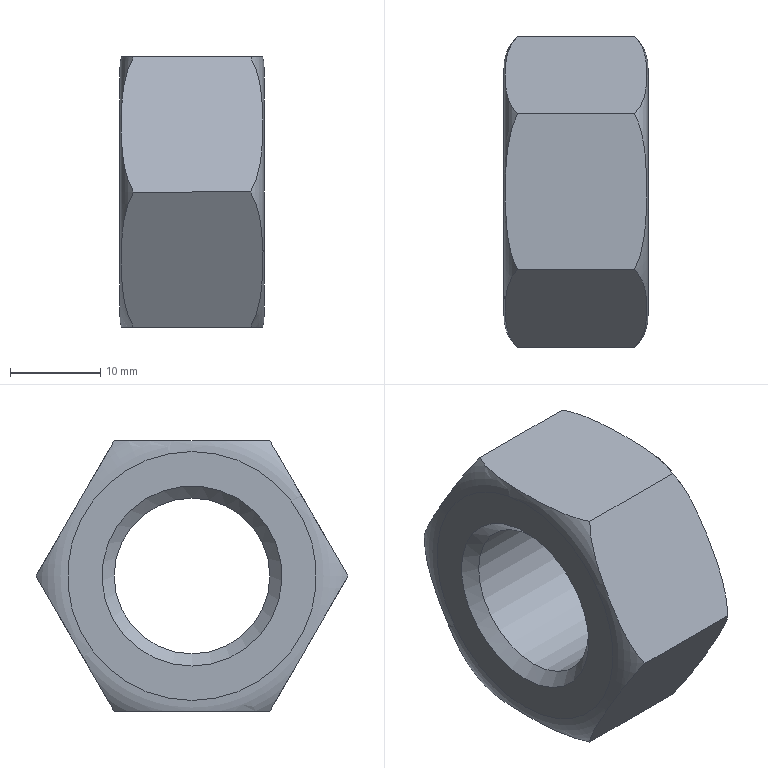Part | STEP file | C-CFJFNV60-20-150_n | 1 solid | 13 faces | box 16 x 34.641 x 30 mm | volume 8537 mm3 | plane 8 | torus 2 | cone 2 | cylinder 1 | commonest cylinder face diameters 17.294 x1
STEP:
#1=CARTESIAN_POINT('',(-6.5,8.66,15.));
#2=VERTEX_POINT('',#1);
#3=CARTESIAN_POINT('',(-7.854,0.,15.));
#4=VERTEX_POINT('',#3);
#5=CARTESIAN_POINT('',(-6.5,8.66,15.));
#6=CARTESIAN_POINT('',(-6.609,8.453,15.));
#7=CARTESIAN_POINT('',(-6.705,8.244,15.));
#8=CARTESIAN_POINT('',(-7.285,6.855,15.));
#9=CARTESIAN_POINT('',(-7.54,5.487,15.));
#10=CARTESIAN_POINT('',(-7.821,2.703,15.));
#11=CARTESIAN_POINT('',(-7.854,1.288,15.));
#12=CARTESIAN_POINT('',(-7.854,0.,15.));
#13=B_SPLINE_CURVE_WITH_KNOTS('',3,(#5,#6,#7,#8,#9,#10,#11,#12),.UNSPECIFIED.,.F.,.F.,(4,2,2,4),(4.146,4.211,4.598,4.984),.UNSPECIFIED.);
#14=EDGE_CURVE('',#2,#4,#13,.T.);
#15=ORIENTED_EDGE('',*,*,#14,.F.);
#16=CARTESIAN_POINT('',(-6.5,17.321,0.));
#17=VERTEX_POINT('',#16);
#18=CARTESIAN_POINT('',(-6.5,17.321,0.));
#19=CARTESIAN_POINT('',(-6.609,17.217,0.1798));
#20=CARTESIAN_POINT('',(-6.705,17.112,0.3609));
#21=CARTESIAN_POINT('',(-7.285,16.418,1.564));
#22=CARTESIAN_POINT('',(-7.54,15.734,2.748));
#23=CARTESIAN_POINT('',(-7.821,14.342,5.159));
#24=CARTESIAN_POINT('',(-7.854,13.634,6.385));
#25=CARTESIAN_POINT('',(-7.854,12.99,7.5));
#26=CARTESIAN_POINT('',(-7.854,12.346,8.615));
#27=CARTESIAN_POINT('',(-7.821,11.639,9.841));
#28=CARTESIAN_POINT('',(-7.54,10.247,12.252));
#29=CARTESIAN_POINT('',(-7.285,9.563,13.436));
#30=CARTESIAN_POINT('',(-6.705,8.869,14.639));
#31=CARTESIAN_POINT('',(-6.609,8.764,14.82));
#32=CARTESIAN_POINT('',(-6.5,8.66,15.));
#33=B_SPLINE_CURVE_WITH_KNOTS('',3,(#18,#19,#20,#21,#22,#23,#24,#25,#26,#27,#28,#29,#30,#31,#32),.UNSPECIFIED.,.F.,.F.,(4,2,2,3,2,2,4),(4.146,4.211,4.598,4.984,5.37,5.757,5.822),.UNSPECIFIED.);
#34=EDGE_CURVE('',#17,#2,#33,.T.);
#35=ORIENTED_EDGE('',*,*,#34,.F.);
#36=CARTESIAN_POINT('',(-6.5,8.66,-15.));
#37=VERTEX_POINT('',#36);
#38=CARTESIAN_POINT('',(-6.5,8.66,-15.));
#39=CARTESIAN_POINT('',(-6.609,8.764,-14.82));
#40=CARTESIAN_POINT('',(-6.705,8.869,-14.639));
#41=CARTESIAN_POINT('',(-7.285,9.563,-13.436));
#42=CARTESIAN_POINT('',(-7.54,10.247,-12.252));
#43=CARTESIAN_POINT('',(-7.821,11.639,-9.841));
#44=CARTESIAN_POINT('',(-7.854,12.346,-8.615));
#45=CARTESIAN_POINT('',(-7.854,12.99,-7.5));
#46=CARTESIAN_POINT('',(-7.854,13.634,-6.385));
#47=CARTESIAN_POINT('',(-7.821,14.342,-5.159));
#48=CARTESIAN_POINT('',(-7.54,15.734,-2.748));
#49=CARTESIAN_POINT('',(-7.285,16.418,-1.564));
#50=CARTESIAN_POINT('',(-6.705,17.112,-0.3609));
#51=CARTESIAN_POINT('',(-6.609,17.217,-0.1798));
#52=CARTESIAN_POINT('',(-6.5,17.321,0.));
#53=B_SPLINE_CURVE_WITH_KNOTS('',3,(#38,#39,#40,#41,#42,#43,#44,#45,#46,#47,#48,#49,#50,#51,#52),.UNSPECIFIED.,.F.,.F.,(4,2,2,3,2,2,4),(4.146,4.211,4.598,4.984,5.37,5.757,5.822),.UNSPECIFIED.);
#54=EDGE_CURVE('',#37,#17,#53,.T.);
#55=ORIENTED_EDGE('',*,*,#54,.F.);
#56=CARTESIAN_POINT('',(-6.5,-8.66,-15.));
#57=VERTEX_POINT('',#56);
#58=CARTESIAN_POINT('',(-6.5,-8.66,-15.));
#59=CARTESIAN_POINT('',(-6.609,-8.453,-15.));
#60=CARTESIAN_POINT('',(-6.705,-8.244,-15.));
#61=CARTESIAN_POINT('',(-7.285,-6.855,-15.));
#62=CARTESIAN_POINT('',(-7.54,-5.487,-15.));
#63=CARTESIAN_POINT('',(-7.821,-2.703,-15.));
#64=CARTESIAN_POINT('',(-7.854,-1.288,-15.));
#65=CARTESIAN_POINT('',(-7.854,0.,-15.));
#66=CARTESIAN_POINT('',(-7.854,1.288,-15.));
#67=CARTESIAN_POINT('',(-7.821,2.703,-15.));
#68=CARTESIAN_POINT('',(-7.54,5.487,-15.));
#69=CARTESIAN_POINT('',(-7.285,6.855,-15.));
#70=CARTESIAN_POINT('',(-6.705,8.244,-15.));
#71=CARTESIAN_POINT('',(-6.609,8.453,-15.));
#72=CARTESIAN_POINT('',(-6.5,8.66,-15.));
#73=B_SPLINE_CURVE_WITH_KNOTS('',3,(#58,#59,#60,#61,#62,#63,#64,#65,#66,#67,#68,#69,#70,#71,#72),.UNSPECIFIED.,.F.,.F.,(4,2,2,3,2,2,4),(4.146,4.211,4.598,4.984,5.37,5.757,5.822),.UNSPECIFIED.);
#74=EDGE_CURVE('',#57,#37,#73,.T.);
#75=ORIENTED_EDGE('',*,*,#74,.F.);
#76=CARTESIAN_POINT('',(-6.5,-17.321,0.));
#77=VERTEX_POINT('',#76);
#78=CARTESIAN_POINT('',(-6.5,-17.321,0.));
#79=CARTESIAN_POINT('',(-6.609,-17.217,-0.1798));
#80=CARTESIAN_POINT('',(-6.705,-17.112,-0.3609));
#81=CARTESIAN_POINT('',(-7.285,-16.418,-1.564));
#82=CARTESIAN_POINT('',(-7.54,-15.734,-2.748));
#83=CARTESIAN_POINT('',(-7.821,-14.342,-5.159));
#84=CARTESIAN_POINT('',(-7.854,-13.634,-6.385));
#85=CARTESIAN_POINT('',(-7.854,-12.99,-7.5));
#86=CARTESIAN_POINT('',(-7.854,-12.346,-8.615));
#87=CARTESIAN_POINT('',(-7.821,-11.639,-9.841));
#88=CARTESIAN_POINT('',(-7.54,-10.247,-12.252));
#89=CARTESIAN_POINT('',(-7.285,-9.563,-13.436));
#90=CARTESIAN_POINT('',(-6.705,-8.869,-14.639));
#91=CARTESIAN_POINT('',(-6.609,-8.764,-14.82));
#92=CARTESIAN_POINT('',(-6.5,-8.66,-15.));
#93=B_SPLINE_CURVE_WITH_KNOTS('',3,(#78,#79,#80,#81,#82,#83,#84,#85,#86,#87,#88,#89,#90,#91,#92),.UNSPECIFIED.,.F.,.F.,(4,2,2,3,2,2,4),(4.146,4.211,4.598,4.984,5.37,5.757,5.822),.UNSPECIFIED.);
#94=EDGE_CURVE('',#77,#57,#93,.T.);
#95=ORIENTED_EDGE('',*,*,#94,.F.);
#96=CARTESIAN_POINT('',(-6.5,-8.66,15.));
#97=VERTEX_POINT('',#96);
#98=CARTESIAN_POINT('',(-6.5,-8.66,15.));
#99=CARTESIAN_POINT('',(-6.609,-8.764,14.82));
#100=CARTESIAN_POINT('',(-6.705,-8.869,14.639));
#101=CARTESIAN_POINT('',(-7.285,-9.563,13.436));
#102=CARTESIAN_POINT('',(-7.54,-10.247,12.252));
#103=CARTESIAN_POINT('',(-7.821,-11.639,9.841));
#104=CARTESIAN_POINT('',(-7.854,-12.346,8.615));
#105=CARTESIAN_POINT('',(-7.854,-12.99,7.5));
#106=CARTESIAN_POINT('',(-7.854,-13.634,6.385));
#107=CARTESIAN_POINT('',(-7.821,-14.342,5.159));
#108=CARTESIAN_POINT('',(-7.54,-15.734,2.748));
#109=CARTESIAN_POINT('',(-7.285,-16.418,1.564));
#110=CARTESIAN_POINT('',(-6.705,-17.112,0.3609));
#111=CARTESIAN_POINT('',(-6.609,-17.217,0.1798));
#112=CARTESIAN_POINT('',(-6.5,-17.321,0.));
#113=B_SPLINE_CURVE_WITH_KNOTS('',3,(#98,#99,#100,#101,#102,#103,#104,#105,#106,#107,#108,#109,#110,#111,#112),.UNSPECIFIED.,.F.,.F.,(4,2,2,3,2,2,4),(4.146,4.211,4.598,4.984,5.37,5.757,5.822),.UNSPECIFIED.);
#114=EDGE_CURVE('',#97,#77,#113,.T.);
#115=ORIENTED_EDGE('',*,*,#114,.F.);
#116=CARTESIAN_POINT('',(-7.854,0.,15.));
#117=CARTESIAN_POINT('',(-7.854,-1.288,15.));
#118=CARTESIAN_POINT('',(-7.821,-2.703,15.));
#119=CARTESIAN_POINT('',(-7.54,-5.487,15.));
#120=CARTESIAN_POINT('',(-7.285,-6.855,15.));
#121=CARTESIAN_POINT('',(-6.705,-8.244,15.));
#122=CARTESIAN_POINT('',(-6.609,-8.453,15.));
#123=CARTESIAN_POINT('',(-6.5,-8.66,15.));
#124=B_SPLINE_CURVE_WITH_KNOTS('',3,(#116,#117,#118,#119,#120,#121,#122,#123),.UNSPECIFIED.,.F.,.F.,(4,2,2,4),(4.984,5.37,5.757,5.822),.UNSPECIFIED.);
#125=EDGE_CURVE('',#4,#97,#124,.T.);
#126=ORIENTED_EDGE('',*,*,#125,.F.);
#127=CARTESIAN_POINT('',(-8.,0.,13.821));
#128=VERTEX_POINT('',#127);
#129=CARTESIAN_POINT('',(-3.167,0.,13.821));
#130=DIRECTION('',(0.,-1.,0.));
#131=DIRECTION('',(0.,0.,1.));
#132=AXIS2_PLACEMENT_3D('',#129,#130,#131);
#133=CIRCLE('',#132,4.833);
#134=EDGE_CURVE('',#4,#128,#133,.T.);
#135=ORIENTED_EDGE('',*,*,#134,.T.);
#136=CARTESIAN_POINT('',(-8.,0.,-13.821));
#137=VERTEX_POINT('',#136);
#138=CARTESIAN_POINT('',(-8.,0.,0.));
#139=DIRECTION('',(1.,0.,0.));
#140=DIRECTION('',(0.,0.,-1.));
#141=AXIS2_PLACEMENT_3D('',#138,#139,#140);
#142=CIRCLE('',#141,13.821);
#143=EDGE_CURVE('',#128,#137,#142,.T.);
#144=ORIENTED_EDGE('',*,*,#143,.T.);
#145=CARTESIAN_POINT('',(-8.,0.,0.));
#146=DIRECTION('',(1.,0.,0.));
#147=DIRECTION('',(0.,0.,-1.));
#148=AXIS2_PLACEMENT_3D('',#145,#146,#147);
#149=CIRCLE('',#148,13.821);
#150=EDGE_CURVE('',#137,#128,#149,.T.);
#151=ORIENTED_EDGE('',*,*,#150,.T.);
#152=ORIENTED_EDGE('',*,*,#134,.F.);
#153=EDGE_LOOP('',(#15,#35,#55,#75,#95,#115,#126,#135,#144,#151,#152));
#154=FACE_OUTER_BOUND('',#153,.T.);
#155=CARTESIAN_POINT('',(-3.167,0.,0.));
#156=DIRECTION('',(1.,0.,0.));
#157=DIRECTION('',(0.,0.,-1.));
#158=AXIS2_PLACEMENT_3D('',#155,#156,#157);
#159=TOROIDAL_SURFACE('',#158,13.821,4.833);
#160=ADVANCED_FACE('',(#154),#159,.T.);
#161=ORIENTED_EDGE('',*,*,#150,.F.);
#162=ORIENTED_EDGE('',*,*,#143,.F.);
#163=EDGE_LOOP('',(#161,#162));
#164=FACE_OUTER_BOUND('',#163,.T.);
#165=CARTESIAN_POINT('',(-8.,0.,-10.));
#166=VERTEX_POINT('',#165);
#167=CARTESIAN_POINT('',(-8.,0.,0.));
#168=DIRECTION('',(1.,0.,0.));
#169=DIRECTION('',(0.,0.,-1.));
#170=AXIS2_PLACEMENT_3D('',#167,#168,#169);
#171=CIRCLE('',#170,10.);
#172=EDGE_CURVE('',#166,#166,#171,.T.);
#173=ORIENTED_EDGE('',*,*,#172,.T.);
#174=EDGE_LOOP('',(#173));
#175=FACE_BOUND('',#174,.T.);
#176=CARTESIAN_POINT('',(-8.,13.821,0.));
#177=DIRECTION('',(-1.,0.,0.));
#178=DIRECTION('',(0.,0.,1.));
#179=AXIS2_PLACEMENT_3D('',#176,#177,#178);
#180=PLANE('',#179);
#181=ADVANCED_FACE('',(#164,#175),#180,.T.);
#182=CARTESIAN_POINT('',(-6.647,0.,-8.647));
#183=VERTEX_POINT('',#182);
#184=CARTESIAN_POINT('',(-6.647,0.,8.647));
#185=VERTEX_POINT('',#184);
#186=CARTESIAN_POINT('',(-6.647,0.,0.));
#187=DIRECTION('',(1.,0.,0.));
#188=DIRECTION('',(0.,0.,-1.));
#189=AXIS2_PLACEMENT_3D('',#186,#187,#188);
#190=CIRCLE('',#189,8.647);
#191=EDGE_CURVE('',#183,#185,#190,.T.);
#192=ORIENTED_EDGE('',*,*,#191,.T.);
#193=CARTESIAN_POINT('',(-6.647,0.,0.));
#194=DIRECTION('',(1.,0.,0.));
#195=DIRECTION('',(0.,0.,-1.));
#196=AXIS2_PLACEMENT_3D('',#193,#194,#195);
#197=CIRCLE('',#196,8.647);
#198=EDGE_CURVE('',#185,#183,#197,.T.);
#199=ORIENTED_EDGE('',*,*,#198,.T.);
#200=CARTESIAN_POINT('',(-8.,0.,-10.));
#201=DIRECTION('',(-0.7071,0.,-0.7071));
#202=VECTOR('',#201,10.);
#203=LINE('',#200,#202);
#204=EDGE_CURVE('',#183,#166,#203,.T.);
#205=ORIENTED_EDGE('',*,*,#204,.T.);
#206=ORIENTED_EDGE('',*,*,#172,.F.);
#207=ORIENTED_EDGE('',*,*,#204,.F.);
#208=EDGE_LOOP('',(#192,#199,#205,#206,#207));
#209=FACE_OUTER_BOUND('',#208,.T.);
#210=CARTESIAN_POINT('',(-8.,0.,0.));
#211=DIRECTION('',(-1.,0.,0.));
#212=DIRECTION('',(0.,0.,1.));
#213=AXIS2_PLACEMENT_3D('',#210,#211,#212);
#214=CONICAL_SURFACE('',#213,10.,0.7854);
#215=ADVANCED_FACE('',(#209),#214,.F.);
#216=ORIENTED_EDGE('',*,*,#191,.F.);
#217=ORIENTED_EDGE('',*,*,#198,.F.);
#218=CARTESIAN_POINT('',(6.647,0.,8.647));
#219=VERTEX_POINT('',#218);
#220=CARTESIAN_POINT('',(8.,0.,8.647));
#221=DIRECTION('',(1.,0.,0.));
#222=VECTOR('',#221,8.647);
#223=LINE('',#220,#222);
#224=EDGE_CURVE('',#185,#219,#223,.T.);
#225=ORIENTED_EDGE('',*,*,#224,.T.);
#226=CARTESIAN_POINT('',(6.647,0.,-8.647));
#227=VERTEX_POINT('',#226);
#228=CARTESIAN_POINT('',(6.647,0.,0.));
#229=DIRECTION('',(1.,0.,0.));
#230=DIRECTION('',(0.,0.,-1.));
#231=AXIS2_PLACEMENT_3D('',#228,#229,#230);
#232=CIRCLE('',#231,8.647);
#233=EDGE_CURVE('',#219,#227,#232,.T.);
#234=ORIENTED_EDGE('',*,*,#233,.T.);
#235=CARTESIAN_POINT('',(6.647,0.,0.));
#236=DIRECTION('',(1.,0.,0.));
#237=DIRECTION('',(0.,0.,-1.));
#238=AXIS2_PLACEMENT_3D('',#235,#236,#237);
#239=CIRCLE('',#238,8.647);
#240=EDGE_CURVE('',#227,#219,#239,.T.);
#241=ORIENTED_EDGE('',*,*,#240,.T.);
#242=ORIENTED_EDGE('',*,*,#224,.F.);
#243=EDGE_LOOP('',(#216,#217,#225,#234,#241,#242));
#244=FACE_OUTER_BOUND('',#243,.T.);
#245=CARTESIAN_POINT('',(8.,0.,0.));
#246=DIRECTION('',(1.,0.,0.));
#247=DIRECTION('',(0.,0.,-1.));
#248=AXIS2_PLACEMENT_3D('',#245,#246,#247);
#249=CYLINDRICAL_SURFACE('',#248,8.647);
#250=ADVANCED_FACE('',(#244),#249,.F.);
#251=ORIENTED_EDGE('',*,*,#240,.F.);
#252=ORIENTED_EDGE('',*,*,#233,.F.);
#253=CARTESIAN_POINT('',(8.,0.,10.));
#254=VERTEX_POINT('',#253);
#255=CARTESIAN_POINT('',(6.647,0.,8.647));
#256=DIRECTION('',(0.7071,0.,0.7071));
#257=VECTOR('',#256,8.647);
#258=LINE('',#255,#257);
#259=EDGE_CURVE('',#219,#254,#258,.T.);
#260=ORIENTED_EDGE('',*,*,#259,.T.);
#261=CARTESIAN_POINT('',(8.,0.,-10.));
#262=VERTEX_POINT('',#261);
#263=CARTESIAN_POINT('',(8.,0.,0.));
#264=DIRECTION('',(1.,0.,0.));
#265=DIRECTION('',(0.,0.,-1.));
#266=AXIS2_PLACEMENT_3D('',#263,#264,#265);
#267=CIRCLE('',#266,10.);
#268=EDGE_CURVE('',#254,#262,#267,.T.);
#269=ORIENTED_EDGE('',*,*,#268,.T.);
#270=CARTESIAN_POINT('',(8.,0.,0.));
#271=DIRECTION('',(1.,0.,0.));
#272=DIRECTION('',(0.,0.,-1.));
#273=AXIS2_PLACEMENT_3D('',#270,#271,#272);
#274=CIRCLE('',#273,10.);
#275=EDGE_CURVE('',#262,#254,#274,.T.);
#276=ORIENTED_EDGE('',*,*,#275,.T.);
#277=ORIENTED_EDGE('',*,*,#259,.F.);
#278=EDGE_LOOP('',(#251,#252,#260,#269,#276,#277));
#279=FACE_OUTER_BOUND('',#278,.T.);
#280=CARTESIAN_POINT('',(6.647,0.,0.));
#281=DIRECTION('',(1.,0.,0.));
#282=DIRECTION('',(0.,0.,-1.));
#283=AXIS2_PLACEMENT_3D('',#280,#281,#282);
#284=CONICAL_SURFACE('',#283,8.647,0.7854);
#285=ADVANCED_FACE('',(#279),#284,.F.);
#286=CARTESIAN_POINT('',(8.,0.,-13.821));
#287=VERTEX_POINT('',#286);
#288=CARTESIAN_POINT('',(8.,0.,13.821));
#289=VERTEX_POINT('',#288);
#290=CARTESIAN_POINT('',(8.,0.,0.));
#291=DIRECTION('',(1.,0.,0.));
#292=DIRECTION('',(0.,0.,-1.));
#293=AXIS2_PLACEMENT_3D('',#290,#291,#292);
#294=CIRCLE('',#293,13.821);
#295=EDGE_CURVE('',#287,#289,#294,.T.);
#296=ORIENTED_EDGE('',*,*,#295,.T.);
#297=CARTESIAN_POINT('',(8.,0.,0.));
#298=DIRECTION('',(1.,0.,0.));
#299=DIRECTION('',(0.,0.,-1.));
#300=AXIS2_PLACEMENT_3D('',#297,#298,#299);
#301=CIRCLE('',#300,13.821);
#302=EDGE_CURVE('',#289,#287,#301,.T.);
#303=ORIENTED_EDGE('',*,*,#302,.T.);
#304=EDGE_LOOP('',(#296,#303));
#305=FACE_OUTER_BOUND('',#304,.T.);
#306=ORIENTED_EDGE('',*,*,#275,.F.);
#307=ORIENTED_EDGE('',*,*,#268,.F.);
#308=EDGE_LOOP('',(#306,#307));
#309=FACE_BOUND('',#308,.T.);
#310=CARTESIAN_POINT('',(8.,10.,0.));
#311=DIRECTION('',(1.,0.,0.));
#312=DIRECTION('',(0.,0.,-1.));
#313=AXIS2_PLACEMENT_3D('',#310,#311,#312);
#314=PLANE('',#313);
#315=ADVANCED_FACE('',(#305,#309),#314,.T.);
#316=ORIENTED_EDGE('',*,*,#295,.F.);
#317=ORIENTED_EDGE('',*,*,#302,.F.);
#318=CARTESIAN_POINT('',(7.854,0.,15.));
#319=VERTEX_POINT('',#318);
#320=CARTESIAN_POINT('',(3.167,0.,13.821));
#321=DIRECTION('',(0.,-1.,0.));
#322=DIRECTION('',(0.,0.,1.));
#323=AXIS2_PLACEMENT_3D('',#320,#321,#322);
#324=CIRCLE('',#323,4.833);
#325=EDGE_CURVE('',#289,#319,#324,.T.);
#326=ORIENTED_EDGE('',*,*,#325,.T.);
#327=CARTESIAN_POINT('',(6.5,-8.66,15.));
#328=VERTEX_POINT('',#327);
#329=CARTESIAN_POINT('',(6.5,-8.66,15.));
#330=CARTESIAN_POINT('',(6.609,-8.453,15.));
#331=CARTESIAN_POINT('',(6.705,-8.244,15.));
#332=CARTESIAN_POINT('',(7.285,-6.855,15.));
#333=CARTESIAN_POINT('',(7.54,-5.487,15.));
#334=CARTESIAN_POINT('',(7.821,-2.703,15.));
#335=CARTESIAN_POINT('',(7.854,-1.288,15.));
#336=CARTESIAN_POINT('',(7.854,0.,15.));
#337=B_SPLINE_CURVE_WITH_KNOTS('',3,(#329,#330,#331,#332,#333,#334,#335,#336),.UNSPECIFIED.,.F.,.F.,(4,2,2,4),(1.654,1.719,2.106,2.492),.UNSPECIFIED.);
#338=EDGE_CURVE('',#328,#319,#337,.T.);
#339=ORIENTED_EDGE('',*,*,#338,.F.);
#340=CARTESIAN_POINT('',(6.5,-17.321,0.));
#341=VERTEX_POINT('',#340);
#342=CARTESIAN_POINT('',(6.5,-17.321,0.));
#343=CARTESIAN_POINT('',(6.609,-17.217,0.1798));
#344=CARTESIAN_POINT('',(6.705,-17.112,0.3609));
#345=CARTESIAN_POINT('',(7.285,-16.418,1.564));
#346=CARTESIAN_POINT('',(7.54,-15.734,2.748));
#347=CARTESIAN_POINT('',(7.821,-14.342,5.159));
#348=CARTESIAN_POINT('',(7.854,-13.634,6.385));
#349=CARTESIAN_POINT('',(7.854,-12.346,8.615));
#350=CARTESIAN_POINT('',(7.821,-11.639,9.841));
#351=CARTESIAN_POINT('',(7.54,-10.247,12.252));
#352=CARTESIAN_POINT('',(7.285,-9.563,13.436));
#353=CARTESIAN_POINT('',(6.705,-8.869,14.639));
#354=CARTESIAN_POINT('',(6.609,-8.764,14.82));
#355=CARTESIAN_POINT('',(6.5,-8.66,15.));
#356=B_SPLINE_CURVE_WITH_KNOTS('',3,(#342,#343,#344,#345,#346,#347,#348,#349,#350,#351,#352,#353,#354,#355),.UNSPECIFIED.,.F.,.F.,(4,2,2,2,2,2,4),(1.654,1.719,2.106,2.492,2.878,3.265,3.33),.UNSPECIFIED.);
#357=EDGE_CURVE('',#341,#328,#356,.T.);
#358=ORIENTED_EDGE('',*,*,#357,.F.);
#359=CARTESIAN_POINT('',(6.5,-8.66,-15.));
#360=VERTEX_POINT('',#359);
#361=CARTESIAN_POINT('',(6.5,-8.66,-15.));
#362=CARTESIAN_POINT('',(6.609,-8.764,-14.82));
#363=CARTESIAN_POINT('',(6.705,-8.869,-14.639));
#364=CARTESIAN_POINT('',(7.285,-9.563,-13.436));
#365=CARTESIAN_POINT('',(7.54,-10.247,-12.252));
#366=CARTESIAN_POINT('',(7.821,-11.639,-9.841));
#367=CARTESIAN_POINT('',(7.854,-12.346,-8.615));
#368=CARTESIAN_POINT('',(7.854,-13.634,-6.385));
#369=CARTESIAN_POINT('',(7.821,-14.342,-5.159));
#370=CARTESIAN_POINT('',(7.54,-15.734,-2.748));
#371=CARTESIAN_POINT('',(7.285,-16.418,-1.564));
#372=CARTESIAN_POINT('',(6.705,-17.112,-0.3609));
#373=CARTESIAN_POINT('',(6.609,-17.217,-0.1798));
#374=CARTESIAN_POINT('',(6.5,-17.321,0.));
#375=B_SPLINE_CURVE_WITH_KNOTS('',3,(#361,#362,#363,#364,#365,#366,#367,#368,#369,#370,#371,#372,#373,#374),.UNSPECIFIED.,.F.,.F.,(4,2,2,2,2,2,4),(1.654,1.719,2.106,2.492,2.878,3.265,3.33),.UNSPECIFIED.);
#376=EDGE_CURVE('',#360,#341,#375,.T.);
#377=ORIENTED_EDGE('',*,*,#376,.F.);
#378=CARTESIAN_POINT('',(6.5,8.66,-15.));
#379=VERTEX_POINT('',#378);
#380=CARTESIAN_POINT('',(6.5,8.66,-15.));
#381=CARTESIAN_POINT('',(6.609,8.453,-15.));
#382=CARTESIAN_POINT('',(6.705,8.244,-15.));
#383=CARTESIAN_POINT('',(7.285,6.855,-15.));
#384=CARTESIAN_POINT('',(7.54,5.487,-15.));
#385=CARTESIAN_POINT('',(7.821,2.703,-15.));
#386=CARTESIAN_POINT('',(7.854,1.288,-15.));
#387=CARTESIAN_POINT('',(7.854,-1.288,-15.));
#388=CARTESIAN_POINT('',(7.821,-2.703,-15.));
#389=CARTESIAN_POINT('',(7.54,-5.487,-15.));
#390=CARTESIAN_POINT('',(7.285,-6.855,-15.));
#391=CARTESIAN_POINT('',(6.705,-8.244,-15.));
#392=CARTESIAN_POINT('',(6.609,-8.453,-15.));
#393=CARTESIAN_POINT('',(6.5,-8.66,-15.));
#394=B_SPLINE_CURVE_WITH_KNOTS('',3,(#380,#381,#382,#383,#384,#385,#386,#387,#388,#389,#390,#391,#392,#393),.UNSPECIFIED.,.F.,.F.,(4,2,2,2,2,2,4),(1.654,1.719,2.106,2.492,2.878,3.265,3.33),.UNSPECIFIED.);
#395=EDGE_CURVE('',#379,#360,#394,.T.);
#396=ORIENTED_EDGE('',*,*,#395,.F.);
#397=CARTESIAN_POINT('',(6.5,17.321,0.));
#398=VERTEX_POINT('',#397);
#399=CARTESIAN_POINT('',(6.5,17.321,0.));
#400=CARTESIAN_POINT('',(6.609,17.217,-0.1798));
#401=CARTESIAN_POINT('',(6.705,17.112,-0.3609));
#402=CARTESIAN_POINT('',(7.285,16.418,-1.564));
#403=CARTESIAN_POINT('',(7.54,15.734,-2.748));
#404=CARTESIAN_POINT('',(7.821,14.342,-5.159));
#405=CARTESIAN_POINT('',(7.854,13.634,-6.385));
#406=CARTESIAN_POINT('',(7.854,12.346,-8.615));
#407=CARTESIAN_POINT('',(7.821,11.639,-9.841));
#408=CARTESIAN_POINT('',(7.54,10.247,-12.252));
#409=CARTESIAN_POINT('',(7.285,9.563,-13.436));
#410=CARTESIAN_POINT('',(6.705,8.869,-14.639));
#411=CARTESIAN_POINT('',(6.609,8.764,-14.82));
#412=CARTESIAN_POINT('',(6.5,8.66,-15.));
#413=B_SPLINE_CURVE_WITH_KNOTS('',3,(#399,#400,#401,#402,#403,#404,#405,#406,#407,#408,#409,#410,#411,#412),.UNSPECIFIED.,.F.,.F.,(4,2,2,2,2,2,4),(1.654,1.719,2.106,2.492,2.878,3.265,3.33),.UNSPECIFIED.);
#414=EDGE_CURVE('',#398,#379,#413,.T.);
#415=ORIENTED_EDGE('',*,*,#414,.F.);
#416=CARTESIAN_POINT('',(6.5,8.66,15.));
#417=VERTEX_POINT('',#416);
#418=CARTESIAN_POINT('',(6.5,8.66,15.));
#419=CARTESIAN_POINT('',(6.609,8.764,14.82));
#420=CARTESIAN_POINT('',(6.705,8.869,14.639));
#421=CARTESIAN_POINT('',(7.285,9.563,13.436));
#422=CARTESIAN_POINT('',(7.54,10.247,12.252));
#423=CARTESIAN_POINT('',(7.821,11.639,9.841));
#424=CARTESIAN_POINT('',(7.854,12.346,8.615));
#425=CARTESIAN_POINT('',(7.854,13.634,6.385));
#426=CARTESIAN_POINT('',(7.821,14.342,5.159));
#427=CARTESIAN_POINT('',(7.54,15.734,2.748));
#428=CARTESIAN_POINT('',(7.285,16.418,1.564));
#429=CARTESIAN_POINT('',(6.705,17.112,0.3609));
#430=CARTESIAN_POINT('',(6.609,17.217,0.1798));
#431=CARTESIAN_POINT('',(6.5,17.321,0.));
#432=B_SPLINE_CURVE_WITH_KNOTS('',3,(#418,#419,#420,#421,#422,#423,#424,#425,#426,#427,#428,#429,#430,#431),.UNSPECIFIED.,.F.,.F.,(4,2,2,2,2,2,4),(1.654,1.719,2.106,2.492,2.878,3.265,3.33),.UNSPECIFIED.);
#433=EDGE_CURVE('',#417,#398,#432,.T.);
#434=ORIENTED_EDGE('',*,*,#433,.F.);
#435=CARTESIAN_POINT('',(7.854,0.,15.));
#436=CARTESIAN_POINT('',(7.854,1.288,15.));
#437=CARTESIAN_POINT('',(7.821,2.703,15.));
#438=CARTESIAN_POINT('',(7.54,5.487,15.));
#439=CARTESIAN_POINT('',(7.285,6.855,15.));
#440=CARTESIAN_POINT('',(6.705,8.244,15.));
#441=CARTESIAN_POINT('',(6.609,8.453,15.));
#442=CARTESIAN_POINT('',(6.5,8.66,15.));
#443=B_SPLINE_CURVE_WITH_KNOTS('',3,(#435,#436,#437,#438,#439,#440,#441,#442),.UNSPECIFIED.,.F.,.F.,(4,2,2,4),(2.492,2.878,3.265,3.33),.UNSPECIFIED.);
#444=EDGE_CURVE('',#319,#417,#443,.T.);
#445=ORIENTED_EDGE('',*,*,#444,.F.);
#446=ORIENTED_EDGE('',*,*,#325,.F.);
#447=EDGE_LOOP('',(#316,#317,#326,#339,#358,#377,#396,#415,#434,#445,#446));
#448=FACE_OUTER_BOUND('',#447,.T.);
#449=CARTESIAN_POINT('',(3.167,0.,0.));
#450=DIRECTION('',(1.,0.,0.));
#451=DIRECTION('',(0.,0.,-1.));
#452=AXIS2_PLACEMENT_3D('',#449,#450,#451);
#453=TOROIDAL_SURFACE('',#452,13.821,4.833);
#454=ADVANCED_FACE('',(#448),#453,.T.);
#455=ORIENTED_EDGE('',*,*,#14,.T.);
#456=ORIENTED_EDGE('',*,*,#125,.T.);
#457=CARTESIAN_POINT('',(16.,-8.66,15.));
#458=DIRECTION('',(-1.,0.,0.));
#459=VECTOR('',#458,1000.);
#460=LINE('',#457,#459);
#461=EDGE_CURVE('',#328,#97,#460,.T.);
#462=ORIENTED_EDGE('',*,*,#461,.F.);
#463=ORIENTED_EDGE('',*,*,#338,.T.);
#464=ORIENTED_EDGE('',*,*,#444,.T.);
#465=CARTESIAN_POINT('',(16.,8.66,15.));
#466=DIRECTION('',(-1.,0.,0.));
#467=VECTOR('',#466,1000.);
#468=LINE('',#465,#467);
#469=EDGE_CURVE('',#417,#2,#468,.T.);
#470=ORIENTED_EDGE('',*,*,#469,.T.);
#471=EDGE_LOOP('',(#455,#456,#462,#463,#464,#470));
#472=FACE_OUTER_BOUND('',#471,.T.);
#473=CARTESIAN_POINT('',(16.,8.66,15.));
#474=DIRECTION('',(0.,0.,-1.));
#475=DIRECTION('',(-1.,0.,0.));
#476=AXIS2_PLACEMENT_3D('',#473,#474,#475);
#477=PLANE('',#476);
#478=ADVANCED_FACE('',(#472),#477,.F.);
#479=ORIENTED_EDGE('',*,*,#34,.T.);
#480=ORIENTED_EDGE('',*,*,#469,.F.);
#481=ORIENTED_EDGE('',*,*,#433,.T.);
#482=CARTESIAN_POINT('',(16.,17.321,0.));
#483=DIRECTION('',(-1.,0.,0.));
#484=VECTOR('',#483,1000.);
#485=LINE('',#482,#484);
#486=EDGE_CURVE('',#398,#17,#485,.T.);
#487=ORIENTED_EDGE('',*,*,#486,.T.);
#488=EDGE_LOOP('',(#479,#480,#481,#487));
#489=FACE_OUTER_BOUND('',#488,.T.);
#490=CARTESIAN_POINT('',(16.,17.321,0.));
#491=DIRECTION('',(0.,-0.866,-0.5));
#492=DIRECTION('',(0.,0.5,-0.866));
#493=AXIS2_PLACEMENT_3D('',#490,#491,#492);
#494=PLANE('',#493);
#495=ADVANCED_FACE('',(#489),#494,.F.);
#496=ORIENTED_EDGE('',*,*,#54,.T.);
#497=ORIENTED_EDGE('',*,*,#486,.F.);
#498=ORIENTED_EDGE('',*,*,#414,.T.);
#499=CARTESIAN_POINT('',(16.,8.66,-15.));
#500=DIRECTION('',(-1.,0.,0.));
#501=VECTOR('',#500,1000.);
#502=LINE('',#499,#501);
#503=EDGE_CURVE('',#379,#37,#502,.T.);
#504=ORIENTED_EDGE('',*,*,#503,.T.);
#505=EDGE_LOOP('',(#496,#497,#498,#504));
#506=FACE_OUTER_BOUND('',#505,.T.);
#507=CARTESIAN_POINT('',(16.,8.66,-15.));
#508=DIRECTION('',(0.,-0.866,0.5));
#509=DIRECTION('',(0.,-0.5,-0.866));
#510=AXIS2_PLACEMENT_3D('',#507,#508,#509);
#511=PLANE('',#510);
#512=ADVANCED_FACE('',(#506),#511,.F.);
#513=ORIENTED_EDGE('',*,*,#74,.T.);
#514=ORIENTED_EDGE('',*,*,#503,.F.);
#515=ORIENTED_EDGE('',*,*,#395,.T.);
#516=CARTESIAN_POINT('',(16.,-8.66,-15.));
#517=DIRECTION('',(-1.,0.,0.));
#518=VECTOR('',#517,1000.);
#519=LINE('',#516,#518);
#520=EDGE_CURVE('',#360,#57,#519,.T.);
#521=ORIENTED_EDGE('',*,*,#520,.T.);
#522=EDGE_LOOP('',(#513,#514,#515,#521));
#523=FACE_OUTER_BOUND('',#522,.T.);
#524=CARTESIAN_POINT('',(16.,-8.66,-15.));
#525=DIRECTION('',(0.,0.,1.));
#526=DIRECTION('',(1.,0.,0.));
#527=AXIS2_PLACEMENT_3D('',#524,#525,#526);
#528=PLANE('',#527);
#529=ADVANCED_FACE('',(#523),#528,.F.);
#530=ORIENTED_EDGE('',*,*,#94,.T.);
#531=ORIENTED_EDGE('',*,*,#520,.F.);
#532=ORIENTED_EDGE('',*,*,#376,.T.);
#533=CARTESIAN_POINT('',(16.,-17.321,0.));
#534=DIRECTION('',(-1.,0.,0.));
#535=VECTOR('',#534,1000.);
#536=LINE('',#533,#535);
#537=EDGE_CURVE('',#341,#77,#536,.T.);
#538=ORIENTED_EDGE('',*,*,#537,.T.);
#539=EDGE_LOOP('',(#530,#531,#532,#538));
#540=FACE_OUTER_BOUND('',#539,.T.);
#541=CARTESIAN_POINT('',(16.,-17.321,0.));
#542=DIRECTION('',(0.,0.866,0.5));
#543=DIRECTION('',(0.,-0.5,0.866));
#544=AXIS2_PLACEMENT_3D('',#541,#542,#543);
#545=PLANE('',#544);
#546=ADVANCED_FACE('',(#540),#545,.F.);
#547=ORIENTED_EDGE('',*,*,#114,.T.);
#548=ORIENTED_EDGE('',*,*,#537,.F.);
#549=ORIENTED_EDGE('',*,*,#357,.T.);
#550=ORIENTED_EDGE('',*,*,#461,.T.);
#551=EDGE_LOOP('',(#547,#548,#549,#550));
#552=FACE_OUTER_BOUND('',#551,.T.);
#553=CARTESIAN_POINT('',(16.,-8.66,15.));
#554=DIRECTION('',(0.,0.866,-0.5));
#555=DIRECTION('',(0.,0.5,0.866));
#556=AXIS2_PLACEMENT_3D('',#553,#554,#555);
#557=PLANE('',#556);
#558=ADVANCED_FACE('',(#552),#557,.F.);
#559=CLOSED_SHELL('',(#160,#181,#215,#250,#285,#315,#454,#478,#495,#512,#529,#546,#558));
#560=MANIFOLD_SOLID_BREP('',#559);
#561=(LENGTH_UNIT()NAMED_UNIT(*)SI_UNIT(.MILLI.,.METRE.));
#562=UNCERTAINTY_MEASURE_WITH_UNIT(LENGTH_MEASURE(0.01),#561,'','');
#563=(NAMED_UNIT(*)PLANE_ANGLE_UNIT()SI_UNIT($,.RADIAN.));
#564=(NAMED_UNIT(*)SI_UNIT($,.STERADIAN.)SOLID_ANGLE_UNIT());
#565=(GEOMETRIC_REPRESENTATION_CONTEXT(3)GLOBAL_UNCERTAINTY_ASSIGNED_CONTEXT((#562))GLOBAL_UNIT_ASSIGNED_CONTEXT((#561,#563,#564))REPRESENTATION_CONTEXT('',''));
#566=ADVANCED_BREP_SHAPE_REPRESENTATION('',(#560),#565);